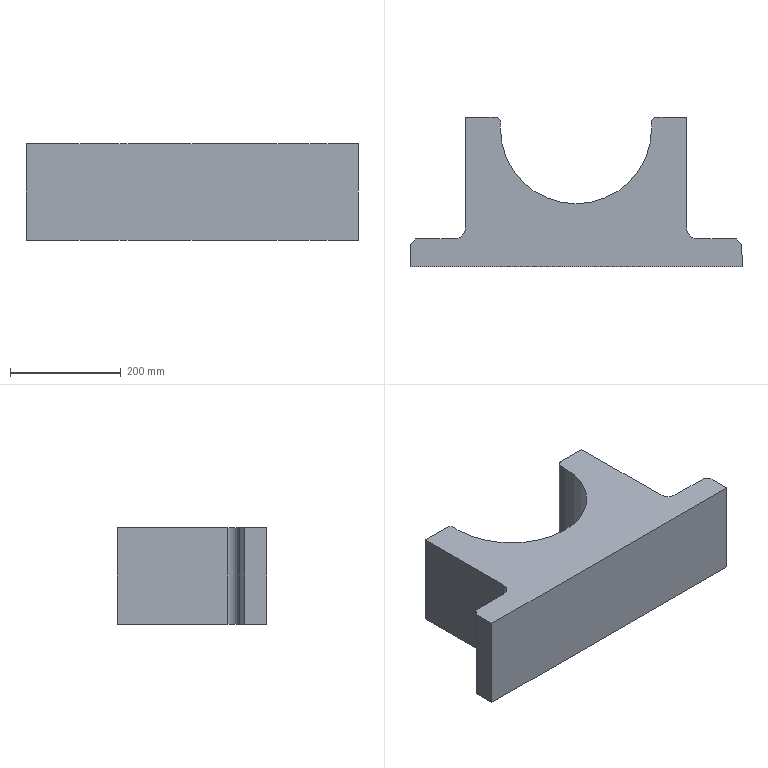Part | SolidWorks | features Fillet 2, Chamfer 1, Extrusion 1, ICE 1, MoveFace 1 | 1 solid | 21 faces | box 600 x 270 x 175 mm | volume 14579348 mm3 | plane 13 | cylinder 8 | commonest cylinder face diameters 20 x3 273 x3 40 x2
STEP:
#1=CARTESIAN_POINT('',(136.158,10.,87.5));
#2=VERTEX_POINT('',#1);
#3=CARTESIAN_POINT('',(136.182,9.317,87.5));
#4=VERTEX_POINT('',#3);
#5=CARTESIAN_POINT('',(146.158,10.,87.5));
#6=DIRECTION('',(0.,0.,1.));
#7=DIRECTION('',(1.,0.,0.));
#8=AXIS2_PLACEMENT_3D('',#5,#6,#7);
#9=CIRCLE('',#8,10.);
#10=EDGE_CURVE('',#2,#4,#9,.T.);
#11=ORIENTED_EDGE('',*,*,#10,.F.);
#12=CARTESIAN_POINT('',(136.158,10.,-87.5));
#13=VERTEX_POINT('',#12);
#14=CARTESIAN_POINT('',(136.158,10.,87.5));
#15=DIRECTION('',(0.,0.,-1.));
#16=VECTOR('',#15,1000.);
#17=LINE('',#14,#16);
#18=EDGE_CURVE('',#2,#13,#17,.T.);
#19=ORIENTED_EDGE('',*,*,#18,.T.);
#20=CARTESIAN_POINT('',(136.182,9.317,-87.5));
#21=VERTEX_POINT('',#20);
#22=CARTESIAN_POINT('',(146.158,10.,-87.5));
#23=DIRECTION('',(0.,0.,-1.));
#24=DIRECTION('',(1.,0.,0.));
#25=AXIS2_PLACEMENT_3D('',#22,#23,#24);
#26=CIRCLE('',#25,10.);
#27=EDGE_CURVE('',#21,#13,#26,.T.);
#28=ORIENTED_EDGE('',*,*,#27,.F.);
#29=CARTESIAN_POINT('',(136.182,9.317,87.5));
#30=DIRECTION('',(0.,0.,-1.));
#31=VECTOR('',#30,1000.);
#32=LINE('',#29,#31);
#33=EDGE_CURVE('',#4,#21,#32,.T.);
#34=ORIENTED_EDGE('',*,*,#33,.F.);
#35=EDGE_LOOP('',(#11,#19,#28,#34));
#36=FACE_OUTER_BOUND('',#35,.T.);
#37=CARTESIAN_POINT('',(146.158,10.,87.5));
#38=DIRECTION('',(0.,0.,-1.));
#39=DIRECTION('',(-1.,0.,0.));
#40=AXIS2_PLACEMENT_3D('',#37,#38,#39);
#41=CYLINDRICAL_SURFACE('',#40,10.);
#42=ADVANCED_FACE('',(#36),#41,.T.);
#43=CARTESIAN_POINT('',(-136.5,0.,87.5));
#44=VERTEX_POINT('',#43);
#45=CARTESIAN_POINT('',(136.5,0.,87.5));
#46=VERTEX_POINT('',#45);
#47=CARTESIAN_POINT('',(0.,0.,87.5));
#48=DIRECTION('',(0.,0.,1.));
#49=DIRECTION('',(1.,0.,0.));
#50=AXIS2_PLACEMENT_3D('',#47,#48,#49);
#51=CIRCLE('',#50,136.5);
#52=EDGE_CURVE('',#44,#46,#51,.T.);
#53=ORIENTED_EDGE('',*,*,#52,.T.);
#54=CARTESIAN_POINT('',(136.5,0.,-87.5));
#55=VERTEX_POINT('',#54);
#56=CARTESIAN_POINT('',(136.5,0.,87.5));
#57=DIRECTION('',(0.,0.,-1.));
#58=VECTOR('',#57,1000.);
#59=LINE('',#56,#58);
#60=EDGE_CURVE('',#46,#55,#59,.T.);
#61=ORIENTED_EDGE('',*,*,#60,.T.);
#62=CARTESIAN_POINT('',(-136.5,0.,-87.5));
#63=VERTEX_POINT('',#62);
#64=CARTESIAN_POINT('',(0.,0.,-87.5));
#65=DIRECTION('',(0.,0.,1.));
#66=DIRECTION('',(1.,0.,0.));
#67=AXIS2_PLACEMENT_3D('',#64,#65,#66);
#68=CIRCLE('',#67,136.5);
#69=EDGE_CURVE('',#63,#55,#68,.T.);
#70=ORIENTED_EDGE('',*,*,#69,.F.);
#71=CARTESIAN_POINT('',(-136.5,0.,87.5));
#72=DIRECTION('',(0.,0.,-1.));
#73=VECTOR('',#72,1000.);
#74=LINE('',#71,#73);
#75=EDGE_CURVE('',#44,#63,#74,.T.);
#76=ORIENTED_EDGE('',*,*,#75,.F.);
#77=EDGE_LOOP('',(#53,#61,#70,#76));
#78=FACE_OUTER_BOUND('',#77,.T.);
#79=CARTESIAN_POINT('',(0.,0.,87.5));
#80=DIRECTION('',(0.,0.,-1.));
#81=DIRECTION('',(-1.,0.,0.));
#82=AXIS2_PLACEMENT_3D('',#79,#80,#81);
#83=CYLINDRICAL_SURFACE('',#82,136.5);
#84=ADVANCED_FACE('',(#78),#83,.F.);
#85=CARTESIAN_POINT('',(-136.182,9.317,87.5));
#86=VERTEX_POINT('',#85);
#87=CARTESIAN_POINT('',(0.,0.,87.5));
#88=DIRECTION('',(0.,0.,1.));
#89=DIRECTION('',(1.,0.,0.));
#90=AXIS2_PLACEMENT_3D('',#87,#88,#89);
#91=CIRCLE('',#90,136.5);
#92=EDGE_CURVE('',#86,#44,#91,.T.);
#93=ORIENTED_EDGE('',*,*,#92,.T.);
#94=ORIENTED_EDGE('',*,*,#75,.T.);
#95=CARTESIAN_POINT('',(-136.182,9.317,-87.5));
#96=VERTEX_POINT('',#95);
#97=CARTESIAN_POINT('',(0.,0.,-87.5));
#98=DIRECTION('',(0.,0.,1.));
#99=DIRECTION('',(1.,0.,0.));
#100=AXIS2_PLACEMENT_3D('',#97,#98,#99);
#101=CIRCLE('',#100,136.5);
#102=EDGE_CURVE('',#96,#63,#101,.T.);
#103=ORIENTED_EDGE('',*,*,#102,.F.);
#104=CARTESIAN_POINT('',(-136.182,9.317,87.5));
#105=DIRECTION('',(0.,0.,1.));
#106=VECTOR('',#105,1000.);
#107=LINE('',#104,#106);
#108=EDGE_CURVE('',#96,#86,#107,.T.);
#109=ORIENTED_EDGE('',*,*,#108,.T.);
#110=EDGE_LOOP('',(#93,#94,#103,#109));
#111=FACE_OUTER_BOUND('',#110,.T.);
#112=CARTESIAN_POINT('',(0.,0.,87.5));
#113=DIRECTION('',(0.,0.,-1.));
#114=DIRECTION('',(-1.,0.,0.));
#115=AXIS2_PLACEMENT_3D('',#112,#113,#114);
#116=CYLINDRICAL_SURFACE('',#115,136.5);
#117=ADVANCED_FACE('',(#111),#116,.F.);
#118=ORIENTED_EDGE('',*,*,#60,.F.);
#119=CARTESIAN_POINT('',(0.,0.,87.5));
#120=DIRECTION('',(0.,0.,1.));
#121=DIRECTION('',(1.,0.,0.));
#122=AXIS2_PLACEMENT_3D('',#119,#120,#121);
#123=CIRCLE('',#122,136.5);
#124=EDGE_CURVE('',#46,#4,#123,.T.);
#125=ORIENTED_EDGE('',*,*,#124,.T.);
#126=ORIENTED_EDGE('',*,*,#33,.T.);
#127=CARTESIAN_POINT('',(0.,0.,-87.5));
#128=DIRECTION('',(0.,0.,1.));
#129=DIRECTION('',(1.,0.,0.));
#130=AXIS2_PLACEMENT_3D('',#127,#128,#129);
#131=CIRCLE('',#130,136.5);
#132=EDGE_CURVE('',#55,#21,#131,.T.);
#133=ORIENTED_EDGE('',*,*,#132,.F.);
#134=EDGE_LOOP('',(#118,#125,#126,#133));
#135=FACE_OUTER_BOUND('',#134,.T.);
#136=CARTESIAN_POINT('',(0.,0.,87.5));
#137=DIRECTION('',(0.,0.,-1.));
#138=DIRECTION('',(-1.,0.,0.));
#139=AXIS2_PLACEMENT_3D('',#136,#137,#138);
#140=CYLINDRICAL_SURFACE('',#139,136.5);
#141=ADVANCED_FACE('',(#135),#140,.F.);
#142=CARTESIAN_POINT('',(300.,-210.,87.5));
#143=VERTEX_POINT('',#142);
#144=CARTESIAN_POINT('',(300.,-250.,87.5));
#145=VERTEX_POINT('',#144);
#146=CARTESIAN_POINT('',(300.,0.,87.5));
#147=DIRECTION('',(0.,-1.,0.));
#148=VECTOR('',#147,1000.);
#149=LINE('',#146,#148);
#150=EDGE_CURVE('',#143,#145,#149,.T.);
#151=ORIENTED_EDGE('',*,*,#150,.F.);
#152=CARTESIAN_POINT('',(290.,-200.,87.5));
#153=VERTEX_POINT('',#152);
#154=CARTESIAN_POINT('',(45.,45.,87.5));
#155=DIRECTION('',(-0.7071,0.7071,0.));
#156=VECTOR('',#155,1000.);
#157=LINE('',#154,#156);
#158=EDGE_CURVE('',#143,#153,#157,.T.);
#159=ORIENTED_EDGE('',*,*,#158,.T.);
#160=CARTESIAN_POINT('',(220.,-200.,87.5));
#161=VERTEX_POINT('',#160);
#162=CARTESIAN_POINT('',(0.,-200.,87.5));
#163=DIRECTION('',(1.,0.,0.));
#164=VECTOR('',#163,1000.);
#165=LINE('',#162,#164);
#166=EDGE_CURVE('',#161,#153,#165,.T.);
#167=ORIENTED_EDGE('',*,*,#166,.F.);
#168=CARTESIAN_POINT('',(200.,-180.,87.5));
#169=VERTEX_POINT('',#168);
#170=CARTESIAN_POINT('',(220.,-180.,87.5));
#171=DIRECTION('',(0.,0.,-1.));
#172=DIRECTION('',(1.,0.,0.));
#173=AXIS2_PLACEMENT_3D('',#170,#171,#172);
#174=CIRCLE('',#173,20.);
#175=EDGE_CURVE('',#161,#169,#174,.T.);
#176=ORIENTED_EDGE('',*,*,#175,.T.);
#177=CARTESIAN_POINT('',(200.,20.,87.5));
#178=VERTEX_POINT('',#177);
#179=CARTESIAN_POINT('',(200.,0.,87.5));
#180=DIRECTION('',(0.,1.,0.));
#181=VECTOR('',#180,1000.);
#182=LINE('',#179,#181);
#183=EDGE_CURVE('',#169,#178,#182,.T.);
#184=ORIENTED_EDGE('',*,*,#183,.T.);
#185=CARTESIAN_POINT('',(146.158,20.,87.5));
#186=VERTEX_POINT('',#185);
#187=CARTESIAN_POINT('',(-200.,20.,87.5));
#188=DIRECTION('',(1.,0.,0.));
#189=VECTOR('',#188,1000.);
#190=LINE('',#187,#189);
#191=EDGE_CURVE('',#186,#178,#190,.T.);
#192=ORIENTED_EDGE('',*,*,#191,.F.);
#193=CARTESIAN_POINT('',(146.158,10.,87.5));
#194=DIRECTION('',(0.,0.,1.));
#195=DIRECTION('',(1.,0.,0.));
#196=AXIS2_PLACEMENT_3D('',#193,#194,#195);
#197=CIRCLE('',#196,10.);
#198=EDGE_CURVE('',#186,#2,#197,.T.);
#199=ORIENTED_EDGE('',*,*,#198,.T.);
#200=ORIENTED_EDGE('',*,*,#10,.T.);
#201=ORIENTED_EDGE('',*,*,#124,.F.);
#202=ORIENTED_EDGE('',*,*,#52,.F.);
#203=ORIENTED_EDGE('',*,*,#92,.F.);
#204=CARTESIAN_POINT('',(-146.158,20.,87.5));
#205=VERTEX_POINT('',#204);
#206=CARTESIAN_POINT('',(-146.158,10.,87.5));
#207=DIRECTION('',(0.,0.,1.));
#208=DIRECTION('',(1.,0.,0.));
#209=AXIS2_PLACEMENT_3D('',#206,#207,#208);
#210=CIRCLE('',#209,10.);
#211=EDGE_CURVE('',#86,#205,#210,.T.);
#212=ORIENTED_EDGE('',*,*,#211,.T.);
#213=CARTESIAN_POINT('',(-200.,20.,87.5));
#214=VERTEX_POINT('',#213);
#215=CARTESIAN_POINT('',(-200.,20.,87.5));
#216=DIRECTION('',(1.,0.,0.));
#217=VECTOR('',#216,1000.);
#218=LINE('',#215,#217);
#219=EDGE_CURVE('',#214,#205,#218,.T.);
#220=ORIENTED_EDGE('',*,*,#219,.F.);
#221=CARTESIAN_POINT('',(-200.,-180.,87.5));
#222=VERTEX_POINT('',#221);
#223=CARTESIAN_POINT('',(-200.,0.,87.5));
#224=DIRECTION('',(0.,1.,0.));
#225=VECTOR('',#224,1000.);
#226=LINE('',#223,#225);
#227=EDGE_CURVE('',#222,#214,#226,.T.);
#228=ORIENTED_EDGE('',*,*,#227,.F.);
#229=CARTESIAN_POINT('',(-220.,-200.,87.5));
#230=VERTEX_POINT('',#229);
#231=CARTESIAN_POINT('',(-220.,-180.,87.5));
#232=DIRECTION('',(0.,0.,-1.));
#233=DIRECTION('',(1.,0.,0.));
#234=AXIS2_PLACEMENT_3D('',#231,#232,#233);
#235=CIRCLE('',#234,20.);
#236=EDGE_CURVE('',#222,#230,#235,.T.);
#237=ORIENTED_EDGE('',*,*,#236,.T.);
#238=CARTESIAN_POINT('',(-290.,-200.,87.5));
#239=VERTEX_POINT('',#238);
#240=CARTESIAN_POINT('',(0.,-200.,87.5));
#241=DIRECTION('',(1.,0.,0.));
#242=VECTOR('',#241,1000.);
#243=LINE('',#240,#242);
#244=EDGE_CURVE('',#239,#230,#243,.T.);
#245=ORIENTED_EDGE('',*,*,#244,.F.);
#246=CARTESIAN_POINT('',(-300.,-210.,87.5));
#247=VERTEX_POINT('',#246);
#248=CARTESIAN_POINT('',(-45.,45.,87.5));
#249=DIRECTION('',(-0.7071,-0.7071,0.));
#250=VECTOR('',#249,1000.);
#251=LINE('',#248,#250);
#252=EDGE_CURVE('',#239,#247,#251,.T.);
#253=ORIENTED_EDGE('',*,*,#252,.T.);
#254=CARTESIAN_POINT('',(-300.,-250.,87.5));
#255=VERTEX_POINT('',#254);
#256=CARTESIAN_POINT('',(-300.,0.,87.5));
#257=DIRECTION('',(0.,-1.,0.));
#258=VECTOR('',#257,1000.);
#259=LINE('',#256,#258);
#260=EDGE_CURVE('',#247,#255,#259,.T.);
#261=ORIENTED_EDGE('',*,*,#260,.T.);
#262=CARTESIAN_POINT('',(0.,-250.,87.5));
#263=DIRECTION('',(1.,0.,0.));
#264=VECTOR('',#263,1000.);
#265=LINE('',#262,#264);
#266=EDGE_CURVE('',#255,#145,#265,.T.);
#267=ORIENTED_EDGE('',*,*,#266,.T.);
#268=EDGE_LOOP('',(#151,#159,#167,#176,#184,#192,#199,#200,#201,#202,#203,#212,#220,#228,#237,#245,#253,#261,#267));
#269=FACE_OUTER_BOUND('',#268,.T.);
#270=CARTESIAN_POINT('',(0.,0.,87.5));
#271=DIRECTION('',(0.,0.,1.));
#272=DIRECTION('',(1.,0.,0.));
#273=AXIS2_PLACEMENT_3D('',#270,#271,#272);
#274=PLANE('',#273);
#275=ADVANCED_FACE('',(#269),#274,.T.);
#276=CARTESIAN_POINT('',(220.,-200.,-87.5));
#277=VERTEX_POINT('',#276);
#278=CARTESIAN_POINT('',(290.,-200.,-87.5));
#279=VERTEX_POINT('',#278);
#280=CARTESIAN_POINT('',(0.,-200.,-87.5));
#281=DIRECTION('',(1.,0.,0.));
#282=VECTOR('',#281,1000.);
#283=LINE('',#280,#282);
#284=EDGE_CURVE('',#277,#279,#283,.T.);
#285=ORIENTED_EDGE('',*,*,#284,.T.);
#286=CARTESIAN_POINT('',(300.,-210.,-87.5));
#287=VERTEX_POINT('',#286);
#288=CARTESIAN_POINT('',(290.,-200.,-87.5));
#289=DIRECTION('',(0.7071,-0.7071,0.));
#290=VECTOR('',#289,1000.);
#291=LINE('',#288,#290);
#292=EDGE_CURVE('',#279,#287,#291,.T.);
#293=ORIENTED_EDGE('',*,*,#292,.T.);
#294=CARTESIAN_POINT('',(300.,-250.,-87.5));
#295=VERTEX_POINT('',#294);
#296=CARTESIAN_POINT('',(300.,0.,-87.5));
#297=DIRECTION('',(0.,-1.,0.));
#298=VECTOR('',#297,1000.);
#299=LINE('',#296,#298);
#300=EDGE_CURVE('',#287,#295,#299,.T.);
#301=ORIENTED_EDGE('',*,*,#300,.T.);
#302=CARTESIAN_POINT('',(-300.,-250.,-87.5));
#303=VERTEX_POINT('',#302);
#304=CARTESIAN_POINT('',(0.,-250.,-87.5));
#305=DIRECTION('',(1.,0.,0.));
#306=VECTOR('',#305,1000.);
#307=LINE('',#304,#306);
#308=EDGE_CURVE('',#303,#295,#307,.T.);
#309=ORIENTED_EDGE('',*,*,#308,.F.);
#310=CARTESIAN_POINT('',(-300.,-210.,-87.5));
#311=VERTEX_POINT('',#310);
#312=CARTESIAN_POINT('',(-300.,0.,-87.5));
#313=DIRECTION('',(0.,-1.,0.));
#314=VECTOR('',#313,1000.);
#315=LINE('',#312,#314);
#316=EDGE_CURVE('',#311,#303,#315,.T.);
#317=ORIENTED_EDGE('',*,*,#316,.F.);
#318=CARTESIAN_POINT('',(-290.,-200.,-87.5));
#319=VERTEX_POINT('',#318);
#320=CARTESIAN_POINT('',(-300.,-210.,-87.5));
#321=DIRECTION('',(0.7071,0.7071,0.));
#322=VECTOR('',#321,1000.);
#323=LINE('',#320,#322);
#324=EDGE_CURVE('',#311,#319,#323,.T.);
#325=ORIENTED_EDGE('',*,*,#324,.T.);
#326=CARTESIAN_POINT('',(-220.,-200.,-87.5));
#327=VERTEX_POINT('',#326);
#328=CARTESIAN_POINT('',(0.,-200.,-87.5));
#329=DIRECTION('',(1.,0.,0.));
#330=VECTOR('',#329,1000.);
#331=LINE('',#328,#330);
#332=EDGE_CURVE('',#319,#327,#331,.T.);
#333=ORIENTED_EDGE('',*,*,#332,.T.);
#334=CARTESIAN_POINT('',(-200.,-180.,-87.5));
#335=VERTEX_POINT('',#334);
#336=CARTESIAN_POINT('',(-220.,-180.,-87.5));
#337=DIRECTION('',(0.,0.,1.));
#338=DIRECTION('',(1.,0.,0.));
#339=AXIS2_PLACEMENT_3D('',#336,#337,#338);
#340=CIRCLE('',#339,20.);
#341=EDGE_CURVE('',#327,#335,#340,.T.);
#342=ORIENTED_EDGE('',*,*,#341,.T.);
#343=CARTESIAN_POINT('',(-200.,20.,-87.5));
#344=VERTEX_POINT('',#343);
#345=CARTESIAN_POINT('',(-200.,0.,-87.5));
#346=DIRECTION('',(0.,1.,0.));
#347=VECTOR('',#346,1000.);
#348=LINE('',#345,#347);
#349=EDGE_CURVE('',#335,#344,#348,.T.);
#350=ORIENTED_EDGE('',*,*,#349,.T.);
#351=CARTESIAN_POINT('',(-146.158,20.,-87.5));
#352=VERTEX_POINT('',#351);
#353=CARTESIAN_POINT('',(0.,20.,-87.5));
#354=DIRECTION('',(-1.,0.,0.));
#355=VECTOR('',#354,1000.);
#356=LINE('',#353,#355);
#357=EDGE_CURVE('',#352,#344,#356,.T.);
#358=ORIENTED_EDGE('',*,*,#357,.F.);
#359=CARTESIAN_POINT('',(-146.158,10.,-87.5));
#360=DIRECTION('',(0.,0.,-1.));
#361=DIRECTION('',(1.,0.,0.));
#362=AXIS2_PLACEMENT_3D('',#359,#360,#361);
#363=CIRCLE('',#362,10.);
#364=EDGE_CURVE('',#352,#96,#363,.T.);
#365=ORIENTED_EDGE('',*,*,#364,.T.);
#366=ORIENTED_EDGE('',*,*,#102,.T.);
#367=ORIENTED_EDGE('',*,*,#69,.T.);
#368=ORIENTED_EDGE('',*,*,#132,.T.);
#369=ORIENTED_EDGE('',*,*,#27,.T.);
#370=CARTESIAN_POINT('',(146.158,20.,-87.5));
#371=VERTEX_POINT('',#370);
#372=CARTESIAN_POINT('',(146.158,10.,-87.5));
#373=DIRECTION('',(0.,0.,-1.));
#374=DIRECTION('',(1.,0.,0.));
#375=AXIS2_PLACEMENT_3D('',#372,#373,#374);
#376=CIRCLE('',#375,10.);
#377=EDGE_CURVE('',#13,#371,#376,.T.);
#378=ORIENTED_EDGE('',*,*,#377,.T.);
#379=CARTESIAN_POINT('',(200.,20.,-87.5));
#380=VERTEX_POINT('',#379);
#381=CARTESIAN_POINT('',(-200.,20.,-87.5));
#382=DIRECTION('',(-1.,0.,0.));
#383=VECTOR('',#382,1000.);
#384=LINE('',#381,#383);
#385=EDGE_CURVE('',#380,#371,#384,.T.);
#386=ORIENTED_EDGE('',*,*,#385,.F.);
#387=CARTESIAN_POINT('',(200.,-180.,-87.5));
#388=VERTEX_POINT('',#387);
#389=CARTESIAN_POINT('',(200.,0.,-87.5));
#390=DIRECTION('',(0.,1.,0.));
#391=VECTOR('',#390,1000.);
#392=LINE('',#389,#391);
#393=EDGE_CURVE('',#388,#380,#392,.T.);
#394=ORIENTED_EDGE('',*,*,#393,.F.);
#395=CARTESIAN_POINT('',(220.,-180.,-87.5));
#396=DIRECTION('',(0.,0.,1.));
#397=DIRECTION('',(1.,0.,0.));
#398=AXIS2_PLACEMENT_3D('',#395,#396,#397);
#399=CIRCLE('',#398,20.);
#400=EDGE_CURVE('',#388,#277,#399,.T.);
#401=ORIENTED_EDGE('',*,*,#400,.T.);
#402=EDGE_LOOP('',(#285,#293,#301,#309,#317,#325,#333,#342,#350,#358,#365,#366,#367,#368,#369,#378,#386,#394,#401));
#403=FACE_OUTER_BOUND('',#402,.T.);
#404=CARTESIAN_POINT('',(0.,0.,-87.5));
#405=DIRECTION('',(0.,0.,1.));
#406=DIRECTION('',(1.,0.,0.));
#407=AXIS2_PLACEMENT_3D('',#404,#405,#406);
#408=PLANE('',#407);
#409=ADVANCED_FACE('',(#403),#408,.F.);
#410=ORIENTED_EDGE('',*,*,#183,.F.);
#411=CARTESIAN_POINT('',(200.,-180.,87.5));
#412=DIRECTION('',(0.,0.,-1.));
#413=VECTOR('',#412,1000.);
#414=LINE('',#411,#413);
#415=EDGE_CURVE('',#169,#388,#414,.T.);
#416=ORIENTED_EDGE('',*,*,#415,.T.);
#417=ORIENTED_EDGE('',*,*,#393,.T.);
#418=CARTESIAN_POINT('',(200.,20.,87.5));
#419=DIRECTION('',(0.,0.,-1.));
#420=VECTOR('',#419,1000.);
#421=LINE('',#418,#420);
#422=EDGE_CURVE('',#178,#380,#421,.T.);
#423=ORIENTED_EDGE('',*,*,#422,.F.);
#424=EDGE_LOOP('',(#410,#416,#417,#423));
#425=FACE_OUTER_BOUND('',#424,.T.);
#426=CARTESIAN_POINT('',(200.,0.,87.5));
#427=DIRECTION('',(-1.,0.,0.));
#428=DIRECTION('',(0.,0.,1.));
#429=AXIS2_PLACEMENT_3D('',#426,#427,#428);
#430=PLANE('',#429);
#431=ADVANCED_FACE('',(#425),#430,.F.);
#432=ORIENTED_EDGE('',*,*,#349,.F.);
#433=CARTESIAN_POINT('',(-200.,-180.,87.5));
#434=DIRECTION('',(0.,0.,1.));
#435=VECTOR('',#434,1000.);
#436=LINE('',#433,#435);
#437=EDGE_CURVE('',#335,#222,#436,.T.);
#438=ORIENTED_EDGE('',*,*,#437,.T.);
#439=ORIENTED_EDGE('',*,*,#227,.T.);
#440=CARTESIAN_POINT('',(-200.,20.,87.5));
#441=DIRECTION('',(0.,0.,-1.));
#442=VECTOR('',#441,1000.);
#443=LINE('',#440,#442);
#444=EDGE_CURVE('',#214,#344,#443,.T.);
#445=ORIENTED_EDGE('',*,*,#444,.T.);
#446=EDGE_LOOP('',(#432,#438,#439,#445));
#447=FACE_OUTER_BOUND('',#446,.T.);
#448=CARTESIAN_POINT('',(-200.,0.,87.5));
#449=DIRECTION('',(-1.,0.,0.));
#450=DIRECTION('',(0.,-1.,0.));
#451=AXIS2_PLACEMENT_3D('',#448,#449,#450);
#452=PLANE('',#451);
#453=ADVANCED_FACE('',(#447),#452,.T.);
#454=ORIENTED_EDGE('',*,*,#332,.F.);
#455=CARTESIAN_POINT('',(-290.,-200.,87.5));
#456=DIRECTION('',(0.,0.,1.));
#457=VECTOR('',#456,1000.);
#458=LINE('',#455,#457);
#459=EDGE_CURVE('',#319,#239,#458,.T.);
#460=ORIENTED_EDGE('',*,*,#459,.T.);
#461=ORIENTED_EDGE('',*,*,#244,.T.);
#462=CARTESIAN_POINT('',(-220.,-200.,-87.5));
#463=DIRECTION('',(0.,0.,-1.));
#464=VECTOR('',#463,1000.);
#465=LINE('',#462,#464);
#466=EDGE_CURVE('',#230,#327,#465,.T.);
#467=ORIENTED_EDGE('',*,*,#466,.T.);
#468=EDGE_LOOP('',(#454,#460,#461,#467));
#469=FACE_OUTER_BOUND('',#468,.T.);
#470=CARTESIAN_POINT('',(0.,-200.,87.5));
#471=DIRECTION('',(0.,1.,0.));
#472=DIRECTION('',(-1.,0.,0.));
#473=AXIS2_PLACEMENT_3D('',#470,#471,#472);
#474=PLANE('',#473);
#475=ADVANCED_FACE('',(#469),#474,.T.);
#476=ORIENTED_EDGE('',*,*,#260,.F.);
#477=CARTESIAN_POINT('',(-300.,-210.,-87.5));
#478=DIRECTION('',(0.,0.,-1.));
#479=VECTOR('',#478,1000.);
#480=LINE('',#477,#479);
#481=EDGE_CURVE('',#247,#311,#480,.T.);
#482=ORIENTED_EDGE('',*,*,#481,.T.);
#483=ORIENTED_EDGE('',*,*,#316,.T.);
#484=CARTESIAN_POINT('',(-300.,-250.,87.5));
#485=DIRECTION('',(0.,0.,-1.));
#486=VECTOR('',#485,1000.);
#487=LINE('',#484,#486);
#488=EDGE_CURVE('',#255,#303,#487,.T.);
#489=ORIENTED_EDGE('',*,*,#488,.F.);
#490=EDGE_LOOP('',(#476,#482,#483,#489));
#491=FACE_OUTER_BOUND('',#490,.T.);
#492=CARTESIAN_POINT('',(-300.,0.,87.5));
#493=DIRECTION('',(1.,0.,0.));
#494=DIRECTION('',(0.,1.,0.));
#495=AXIS2_PLACEMENT_3D('',#492,#493,#494);
#496=PLANE('',#495);
#497=ADVANCED_FACE('',(#491),#496,.F.);
#498=ORIENTED_EDGE('',*,*,#308,.T.);
#499=CARTESIAN_POINT('',(300.,-250.,87.5));
#500=DIRECTION('',(0.,0.,-1.));
#501=VECTOR('',#500,1000.);
#502=LINE('',#499,#501);
#503=EDGE_CURVE('',#145,#295,#502,.T.);
#504=ORIENTED_EDGE('',*,*,#503,.F.);
#505=ORIENTED_EDGE('',*,*,#266,.F.);
#506=ORIENTED_EDGE('',*,*,#488,.T.);
#507=EDGE_LOOP('',(#498,#504,#505,#506));
#508=FACE_OUTER_BOUND('',#507,.T.);
#509=CARTESIAN_POINT('',(0.,-250.,87.5));
#510=DIRECTION('',(0.,1.,0.));
#511=DIRECTION('',(-1.,0.,0.));
#512=AXIS2_PLACEMENT_3D('',#509,#510,#511);
#513=PLANE('',#512);
#514=ADVANCED_FACE('',(#508),#513,.F.);
#515=ORIENTED_EDGE('',*,*,#300,.F.);
#516=CARTESIAN_POINT('',(300.,-210.,87.5));
#517=DIRECTION('',(0.,0.,1.));
#518=VECTOR('',#517,1000.);
#519=LINE('',#516,#518);
#520=EDGE_CURVE('',#287,#143,#519,.T.);
#521=ORIENTED_EDGE('',*,*,#520,.T.);
#522=ORIENTED_EDGE('',*,*,#150,.T.);
#523=ORIENTED_EDGE('',*,*,#503,.T.);
#524=EDGE_LOOP('',(#515,#521,#522,#523));
#525=FACE_OUTER_BOUND('',#524,.T.);
#526=CARTESIAN_POINT('',(300.,0.,87.5));
#527=DIRECTION('',(1.,0.,0.));
#528=DIRECTION('',(0.,1.,0.));
#529=AXIS2_PLACEMENT_3D('',#526,#527,#528);
#530=PLANE('',#529);
#531=ADVANCED_FACE('',(#525),#530,.T.);
#532=ORIENTED_EDGE('',*,*,#166,.T.);
#533=CARTESIAN_POINT('',(290.,-200.,87.5));
#534=DIRECTION('',(0.,0.,-1.));
#535=VECTOR('',#534,1000.);
#536=LINE('',#533,#535);
#537=EDGE_CURVE('',#153,#279,#536,.T.);
#538=ORIENTED_EDGE('',*,*,#537,.T.);
#539=ORIENTED_EDGE('',*,*,#284,.F.);
#540=CARTESIAN_POINT('',(220.,-200.,87.5));
#541=DIRECTION('',(0.,0.,1.));
#542=VECTOR('',#541,1000.);
#543=LINE('',#540,#542);
#544=EDGE_CURVE('',#277,#161,#543,.T.);
#545=ORIENTED_EDGE('',*,*,#544,.T.);
#546=EDGE_LOOP('',(#532,#538,#539,#545));
#547=FACE_OUTER_BOUND('',#546,.T.);
#548=CARTESIAN_POINT('',(0.,-200.,87.5));
#549=DIRECTION('',(0.,1.,0.));
#550=DIRECTION('',(-1.,0.,0.));
#551=AXIS2_PLACEMENT_3D('',#548,#549,#550);
#552=PLANE('',#551);
#553=ADVANCED_FACE('',(#547),#552,.T.);
#554=ORIENTED_EDGE('',*,*,#219,.T.);
#555=CARTESIAN_POINT('',(-146.158,20.,0.));
#556=DIRECTION('',(0.,0.,-1.));
#557=VECTOR('',#556,1000.);
#558=LINE('',#555,#557);
#559=EDGE_CURVE('',#205,#352,#558,.T.);
#560=ORIENTED_EDGE('',*,*,#559,.T.);
#561=ORIENTED_EDGE('',*,*,#357,.T.);
#562=ORIENTED_EDGE('',*,*,#444,.F.);
#563=EDGE_LOOP('',(#554,#560,#561,#562));
#564=FACE_OUTER_BOUND('',#563,.T.);
#565=CARTESIAN_POINT('',(0.,20.,0.));
#566=DIRECTION('',(0.,1.,0.));
#567=DIRECTION('',(0.,0.,1.));
#568=AXIS2_PLACEMENT_3D('',#565,#566,#567);
#569=PLANE('',#568);
#570=ADVANCED_FACE('',(#564),#569,.T.);
#571=ORIENTED_EDGE('',*,*,#385,.T.);
#572=CARTESIAN_POINT('',(146.158,20.,0.));
#573=DIRECTION('',(0.,0.,1.));
#574=VECTOR('',#573,1000.);
#575=LINE('',#572,#574);
#576=EDGE_CURVE('',#371,#186,#575,.T.);
#577=ORIENTED_EDGE('',*,*,#576,.T.);
#578=ORIENTED_EDGE('',*,*,#191,.T.);
#579=ORIENTED_EDGE('',*,*,#422,.T.);
#580=EDGE_LOOP('',(#571,#577,#578,#579));
#581=FACE_OUTER_BOUND('',#580,.T.);
#582=CARTESIAN_POINT('',(0.,20.,0.));
#583=DIRECTION('',(0.,1.,0.));
#584=DIRECTION('',(0.,0.,1.));
#585=AXIS2_PLACEMENT_3D('',#582,#583,#584);
#586=PLANE('',#585);
#587=ADVANCED_FACE('',(#581),#586,.T.);
#588=ORIENTED_EDGE('',*,*,#18,.F.);
#589=ORIENTED_EDGE('',*,*,#198,.F.);
#590=ORIENTED_EDGE('',*,*,#576,.F.);
#591=ORIENTED_EDGE('',*,*,#377,.F.);
#592=EDGE_LOOP('',(#588,#589,#590,#591));
#593=FACE_OUTER_BOUND('',#592,.T.);
#594=CARTESIAN_POINT('',(146.158,10.,87.5));
#595=DIRECTION('',(0.,0.,-1.));
#596=DIRECTION('',(-1.,0.,0.));
#597=AXIS2_PLACEMENT_3D('',#594,#595,#596);
#598=CYLINDRICAL_SURFACE('',#597,10.);
#599=ADVANCED_FACE('',(#593),#598,.T.);
#600=ORIENTED_EDGE('',*,*,#364,.F.);
#601=ORIENTED_EDGE('',*,*,#559,.F.);
#602=ORIENTED_EDGE('',*,*,#211,.F.);
#603=ORIENTED_EDGE('',*,*,#108,.F.);
#604=EDGE_LOOP('',(#600,#601,#602,#603));
#605=FACE_OUTER_BOUND('',#604,.T.);
#606=CARTESIAN_POINT('',(-146.158,10.,87.5));
#607=DIRECTION('',(0.,0.,-1.));
#608=DIRECTION('',(-1.,0.,0.));
#609=AXIS2_PLACEMENT_3D('',#606,#607,#608);
#610=CYLINDRICAL_SURFACE('',#609,10.);
#611=ADVANCED_FACE('',(#605),#610,.T.);
#612=ORIENTED_EDGE('',*,*,#236,.F.);
#613=ORIENTED_EDGE('',*,*,#437,.F.);
#614=ORIENTED_EDGE('',*,*,#341,.F.);
#615=ORIENTED_EDGE('',*,*,#466,.F.);
#616=EDGE_LOOP('',(#612,#613,#614,#615));
#617=FACE_OUTER_BOUND('',#616,.T.);
#618=CARTESIAN_POINT('',(-220.,-180.,87.5));
#619=DIRECTION('',(0.,0.,1.));
#620=DIRECTION('',(1.,0.,0.));
#621=AXIS2_PLACEMENT_3D('',#618,#619,#620);
#622=CYLINDRICAL_SURFACE('',#621,20.);
#623=ADVANCED_FACE('',(#617),#622,.F.);
#624=ORIENTED_EDGE('',*,*,#175,.F.);
#625=ORIENTED_EDGE('',*,*,#544,.F.);
#626=ORIENTED_EDGE('',*,*,#400,.F.);
#627=ORIENTED_EDGE('',*,*,#415,.F.);
#628=EDGE_LOOP('',(#624,#625,#626,#627));
#629=FACE_OUTER_BOUND('',#628,.T.);
#630=CARTESIAN_POINT('',(220.,-180.,87.5));
#631=DIRECTION('',(0.,0.,-1.));
#632=DIRECTION('',(-1.,0.,0.));
#633=AXIS2_PLACEMENT_3D('',#630,#631,#632);
#634=CYLINDRICAL_SURFACE('',#633,20.);
#635=ADVANCED_FACE('',(#629),#634,.F.);
#636=ORIENTED_EDGE('',*,*,#158,.F.);
#637=ORIENTED_EDGE('',*,*,#520,.F.);
#638=ORIENTED_EDGE('',*,*,#292,.F.);
#639=ORIENTED_EDGE('',*,*,#537,.F.);
#640=EDGE_LOOP('',(#636,#637,#638,#639));
#641=FACE_OUTER_BOUND('',#640,.T.);
#642=CARTESIAN_POINT('',(290.,-200.,87.5));
#643=DIRECTION('',(-0.7071,-0.7071,0.));
#644=DIRECTION('',(0.,0.,-1.));
#645=AXIS2_PLACEMENT_3D('',#642,#643,#644);
#646=PLANE('',#645);
#647=ADVANCED_FACE('',(#641),#646,.F.);
#648=ORIENTED_EDGE('',*,*,#252,.F.);
#649=ORIENTED_EDGE('',*,*,#459,.F.);
#650=ORIENTED_EDGE('',*,*,#324,.F.);
#651=ORIENTED_EDGE('',*,*,#481,.F.);
#652=EDGE_LOOP('',(#648,#649,#650,#651));
#653=FACE_OUTER_BOUND('',#652,.T.);
#654=CARTESIAN_POINT('',(-300.,-210.,87.5));
#655=DIRECTION('',(-0.7071,0.7071,0.));
#656=DIRECTION('',(0.,0.,1.));
#657=AXIS2_PLACEMENT_3D('',#654,#655,#656);
#658=PLANE('',#657);
#659=ADVANCED_FACE('',(#653),#658,.T.);
#660=CLOSED_SHELL('',(#42,#84,#117,#141,#275,#409,#431,#453,#475,#497,#514,#531,#553,#570,#587,#599,#611,#623,#635,#647,#659));
#661=MANIFOLD_SOLID_BREP('',#660);
#662=CARTESIAN_POINT('',(0.,0.,0.));
#663=DIRECTION('',(0.,0.,1.));
#664=DIRECTION('',(1.,0.,0.));
#665=AXIS2_PLACEMENT_3D('',#662,#663,#664);
#666=(LENGTH_UNIT()NAMED_UNIT(*)SI_UNIT(.MILLI.,.METRE.));
#667=UNCERTAINTY_MEASURE_WITH_UNIT(LENGTH_MEASURE(0.00001),#666,'','');
#668=(NAMED_UNIT(*)PLANE_ANGLE_UNIT()SI_UNIT($,.RADIAN.));
#669=(NAMED_UNIT(*)SI_UNIT($,.STERADIAN.)SOLID_ANGLE_UNIT());
#670=(GEOMETRIC_REPRESENTATION_CONTEXT(3)GLOBAL_UNCERTAINTY_ASSIGNED_CONTEXT((#667))GLOBAL_UNIT_ASSIGNED_CONTEXT((#666,#668,#669))REPRESENTATION_CONTEXT('',''));
#671=ADVANCED_BREP_SHAPE_REPRESENTATION('',(#661,#665),#670);